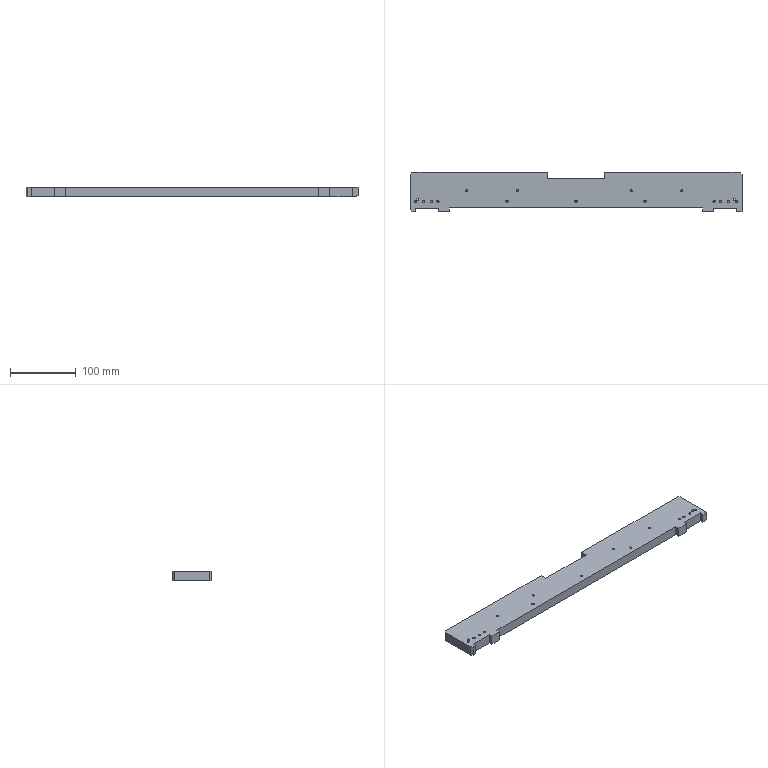Part | STEP file | 11-FG-SZ01811 | 1 solid | 144 faces | box 505 x 60 x 15 mm | volume 395748 mm3 | cylinder 66 | cone 52 | plane 26 | commonest cylinder face diameters 3.3 x38 4.2 x12 4 x8 5 x8